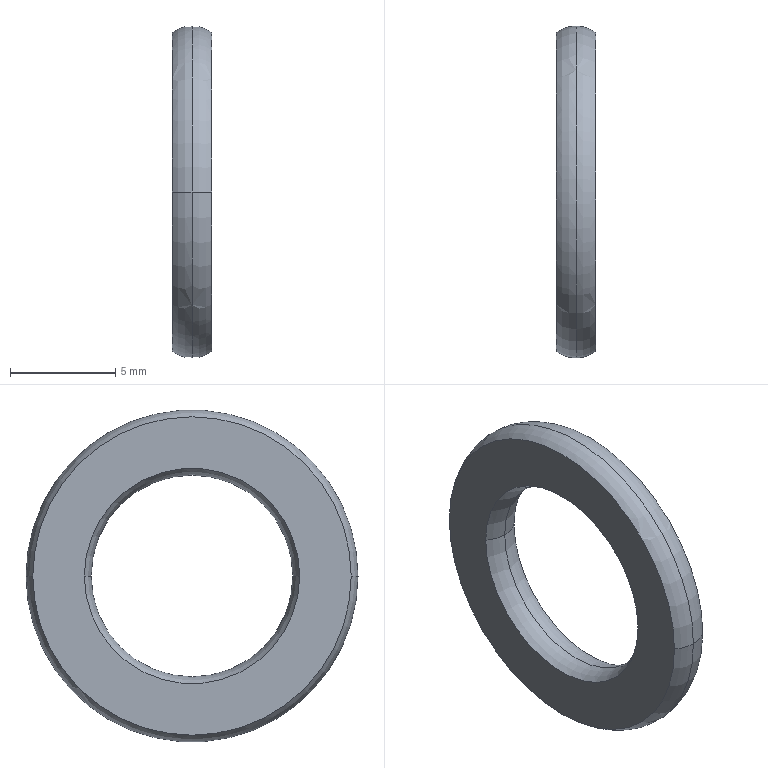Part | Creo | 1 solid | 10 faces | box 1.9 x 15.8 x 15.8 mm | volume 219.321 mm3 | torus 8 | plane 2
STEP:
#1=CARTESIAN_POINT('',(-128.,-90.537,-6.));
#2=VERTEX_POINT('',#1);
#3=CARTESIAN_POINT('',(-128.,-80.286,-6.));
#4=VERTEX_POINT('',#3);
#5=CARTESIAN_POINT('',(-128.,-85.411,-6.));
#6=DIRECTION('',(-1.,0.,0.));
#7=DIRECTION('',(0.,-1.,0.));
#8=AXIS2_PLACEMENT_3D('',#5,#6,#7);
#9=CIRCLE('',#8,5.125);
#10=EDGE_CURVE('',#2,#4,#9,.T.);
#11=ORIENTED_EDGE('',*,*,#10,.T.);
#12=CARTESIAN_POINT('',(-128.95,-80.611,-6.));
#13=VERTEX_POINT('',#12);
#14=CARTESIAN_POINT('',(-128.95,-79.061,-6.));
#15=DIRECTION('',(0.,0.,1.));
#16=DIRECTION('',(0.,-1.,0.));
#17=AXIS2_PLACEMENT_3D('',#14,#15,#16);
#18=CIRCLE('',#17,1.55);
#19=EDGE_CURVE('',#13,#4,#18,.T.);
#20=ORIENTED_EDGE('',*,*,#19,.F.);
#21=CARTESIAN_POINT('',(-128.95,-90.211,-6.));
#22=VERTEX_POINT('',#21);
#23=CARTESIAN_POINT('',(-128.95,-85.411,-6.));
#24=DIRECTION('',(-1.,0.,0.));
#25=DIRECTION('',(0.,-1.,0.));
#26=AXIS2_PLACEMENT_3D('',#23,#24,#25);
#27=CIRCLE('',#26,4.8);
#28=EDGE_CURVE('',#22,#13,#27,.T.);
#29=ORIENTED_EDGE('',*,*,#28,.F.);
#30=CARTESIAN_POINT('',(-128.95,-91.761,-6.));
#31=DIRECTION('',(0.,0.,-1.));
#32=DIRECTION('',(0.,1.,0.));
#33=AXIS2_PLACEMENT_3D('',#30,#31,#32);
#34=CIRCLE('',#33,1.55);
#35=EDGE_CURVE('',#22,#2,#34,.T.);
#36=ORIENTED_EDGE('',*,*,#35,.T.);
#37=EDGE_LOOP('',(#11,#20,#29,#36));
#38=FACE_OUTER_BOUND('',#37,.F.);
#39=CARTESIAN_POINT('',(-128.95,-85.411,-6.));
#40=DIRECTION('',(-1.,0.,0.));
#41=DIRECTION('',(0.,-1.,0.));
#42=AXIS2_PLACEMENT_3D('',#39,#40,#41);
#43=TOROIDAL_SURFACE('',#42,6.35,1.55);
#44=ADVANCED_FACE('',(#38),#43,.T.);
#45=CARTESIAN_POINT('',(-128.,-92.986,-6.));
#46=VERTEX_POINT('',#45);
#47=CARTESIAN_POINT('',(-128.,-77.837,-6.));
#48=VERTEX_POINT('',#47);
#49=CARTESIAN_POINT('',(-128.,-85.411,-6.));
#50=DIRECTION('',(1.,0.,0.));
#51=DIRECTION('',(0.,-1.,0.));
#52=AXIS2_PLACEMENT_3D('',#49,#50,#51);
#53=CIRCLE('',#52,7.575);
#54=EDGE_CURVE('',#46,#48,#53,.T.);
#55=ORIENTED_EDGE('',*,*,#54,.F.);
#56=CARTESIAN_POINT('',(-128.,-85.411,-6.));
#57=DIRECTION('',(1.,0.,0.));
#58=DIRECTION('',(0.,1.,0.));
#59=AXIS2_PLACEMENT_3D('',#56,#57,#58);
#60=CIRCLE('',#59,7.575);
#61=EDGE_CURVE('',#48,#46,#60,.T.);
#62=ORIENTED_EDGE('',*,*,#61,.F.);
#63=EDGE_LOOP('',(#55,#62));
#64=FACE_OUTER_BOUND('',#63,.F.);
#65=ORIENTED_EDGE('',*,*,#10,.F.);
#66=CARTESIAN_POINT('',(-128.,-85.411,-6.));
#67=DIRECTION('',(-1.,0.,0.));
#68=DIRECTION('',(0.,1.,0.));
#69=AXIS2_PLACEMENT_3D('',#66,#67,#68);
#70=CIRCLE('',#69,5.125);
#71=EDGE_CURVE('',#4,#2,#70,.T.);
#72=ORIENTED_EDGE('',*,*,#71,.F.);
#73=EDGE_LOOP('',(#65,#72));
#74=FACE_BOUND('',#73,.F.);
#75=CARTESIAN_POINT('',(-128.,-85.411,1.575));
#76=DIRECTION('',(1.,0.,0.));
#77=DIRECTION('',(0.,1.,0.));
#78=AXIS2_PLACEMENT_3D('',#75,#76,#77);
#79=PLANE('',#78);
#80=ADVANCED_FACE('',(#64,#74),#79,.T.);
#81=ORIENTED_EDGE('',*,*,#71,.T.);
#82=ORIENTED_EDGE('',*,*,#35,.F.);
#83=CARTESIAN_POINT('',(-128.95,-85.411,-6.));
#84=DIRECTION('',(-1.,0.,0.));
#85=DIRECTION('',(0.,1.,0.));
#86=AXIS2_PLACEMENT_3D('',#83,#84,#85);
#87=CIRCLE('',#86,4.8);
#88=EDGE_CURVE('',#13,#22,#87,.T.);
#89=ORIENTED_EDGE('',*,*,#88,.F.);
#90=ORIENTED_EDGE('',*,*,#19,.T.);
#91=EDGE_LOOP('',(#81,#82,#89,#90));
#92=FACE_OUTER_BOUND('',#91,.F.);
#93=CARTESIAN_POINT('',(-128.95,-85.411,-6.));
#94=DIRECTION('',(-1.,0.,0.));
#95=DIRECTION('',(0.,-1.,0.));
#96=AXIS2_PLACEMENT_3D('',#93,#94,#95);
#97=TOROIDAL_SURFACE('',#96,6.35,1.55);
#98=ADVANCED_FACE('',(#92),#97,.T.);
#99=CARTESIAN_POINT('',(-129.9,-90.537,-6.));
#100=VERTEX_POINT('',#99);
#101=CARTESIAN_POINT('',(-129.9,-80.286,-6.));
#102=VERTEX_POINT('',#101);
#103=CARTESIAN_POINT('',(-129.9,-85.411,-6.));
#104=DIRECTION('',(1.,0.,0.));
#105=DIRECTION('',(0.,-1.,0.));
#106=AXIS2_PLACEMENT_3D('',#103,#104,#105);
#107=CIRCLE('',#106,5.125);
#108=EDGE_CURVE('',#100,#102,#107,.T.);
#109=ORIENTED_EDGE('',*,*,#108,.T.);
#110=CARTESIAN_POINT('',(-128.95,-79.061,-6.));
#111=DIRECTION('',(0.,0.,1.));
#112=DIRECTION('',(-0.6129,-0.7902,0.));
#113=AXIS2_PLACEMENT_3D('',#110,#111,#112);
#114=CIRCLE('',#113,1.55);
#115=EDGE_CURVE('',#102,#13,#114,.T.);
#116=ORIENTED_EDGE('',*,*,#115,.T.);
#117=ORIENTED_EDGE('',*,*,#88,.T.);
#118=CARTESIAN_POINT('',(-128.95,-91.761,-6.));
#119=DIRECTION('',(0.,0.,-1.));
#120=DIRECTION('',(-0.6129,0.7902,0.));
#121=AXIS2_PLACEMENT_3D('',#118,#119,#120);
#122=CIRCLE('',#121,1.55);
#123=EDGE_CURVE('',#100,#22,#122,.T.);
#124=ORIENTED_EDGE('',*,*,#123,.F.);
#125=EDGE_LOOP('',(#109,#116,#117,#124));
#126=FACE_OUTER_BOUND('',#125,.F.);
#127=CARTESIAN_POINT('',(-128.95,-85.411,-6.));
#128=DIRECTION('',(-1.,0.,0.));
#129=DIRECTION('',(0.,-1.,0.));
#130=AXIS2_PLACEMENT_3D('',#127,#128,#129);
#131=TOROIDAL_SURFACE('',#130,6.35,1.55);
#132=ADVANCED_FACE('',(#126),#131,.T.);
#133=CARTESIAN_POINT('',(-129.9,-92.986,-6.));
#134=VERTEX_POINT('',#133);
#135=CARTESIAN_POINT('',(-129.9,-77.837,-6.));
#136=VERTEX_POINT('',#135);
#137=CARTESIAN_POINT('',(-129.9,-85.411,-6.));
#138=DIRECTION('',(-1.,0.,0.));
#139=DIRECTION('',(0.,-1.,0.));
#140=AXIS2_PLACEMENT_3D('',#137,#138,#139);
#141=CIRCLE('',#140,7.575);
#142=EDGE_CURVE('',#134,#136,#141,.T.);
#143=ORIENTED_EDGE('',*,*,#142,.F.);
#144=CARTESIAN_POINT('',(-129.9,-85.411,-6.));
#145=DIRECTION('',(-1.,0.,0.));
#146=DIRECTION('',(0.,1.,0.));
#147=AXIS2_PLACEMENT_3D('',#144,#145,#146);
#148=CIRCLE('',#147,7.575);
#149=EDGE_CURVE('',#136,#134,#148,.T.);
#150=ORIENTED_EDGE('',*,*,#149,.F.);
#151=EDGE_LOOP('',(#143,#150));
#152=FACE_OUTER_BOUND('',#151,.F.);
#153=ORIENTED_EDGE('',*,*,#108,.F.);
#154=CARTESIAN_POINT('',(-129.9,-85.411,-6.));
#155=DIRECTION('',(1.,0.,0.));
#156=DIRECTION('',(0.,1.,0.));
#157=AXIS2_PLACEMENT_3D('',#154,#155,#156);
#158=CIRCLE('',#157,5.125);
#159=EDGE_CURVE('',#102,#100,#158,.T.);
#160=ORIENTED_EDGE('',*,*,#159,.F.);
#161=EDGE_LOOP('',(#153,#160));
#162=FACE_BOUND('',#161,.F.);
#163=CARTESIAN_POINT('',(-129.9,-85.411,-0.8749));
#164=DIRECTION('',(-1.,0.,0.));
#165=DIRECTION('',(0.,-1.,0.));
#166=AXIS2_PLACEMENT_3D('',#163,#164,#165);
#167=PLANE('',#166);
#168=ADVANCED_FACE('',(#152,#162),#167,.T.);
#169=ORIENTED_EDGE('',*,*,#142,.T.);
#170=CARTESIAN_POINT('',(-128.95,-77.511,-6.));
#171=VERTEX_POINT('',#170);
#172=CARTESIAN_POINT('',(-128.95,-79.061,-6.));
#173=DIRECTION('',(0.,0.,1.));
#174=DIRECTION('',(0.,1.,0.));
#175=AXIS2_PLACEMENT_3D('',#172,#173,#174);
#176=CIRCLE('',#175,1.55);
#177=EDGE_CURVE('',#171,#136,#176,.T.);
#178=ORIENTED_EDGE('',*,*,#177,.F.);
#179=CARTESIAN_POINT('',(-128.95,-93.311,-6.));
#180=VERTEX_POINT('',#179);
#181=CARTESIAN_POINT('',(-128.95,-85.411,-6.));
#182=DIRECTION('',(-1.,0.,0.));
#183=DIRECTION('',(0.,-1.,0.));
#184=AXIS2_PLACEMENT_3D('',#181,#182,#183);
#185=CIRCLE('',#184,7.9);
#186=EDGE_CURVE('',#180,#171,#185,.T.);
#187=ORIENTED_EDGE('',*,*,#186,.F.);
#188=CARTESIAN_POINT('',(-128.95,-91.761,-6.));
#189=DIRECTION('',(0.,0.,-1.));
#190=DIRECTION('',(0.,-1.,0.));
#191=AXIS2_PLACEMENT_3D('',#188,#189,#190);
#192=CIRCLE('',#191,1.55);
#193=EDGE_CURVE('',#180,#134,#192,.T.);
#194=ORIENTED_EDGE('',*,*,#193,.T.);
#195=EDGE_LOOP('',(#169,#178,#187,#194));
#196=FACE_OUTER_BOUND('',#195,.F.);
#197=CARTESIAN_POINT('',(-128.95,-85.411,-6.));
#198=DIRECTION('',(-1.,0.,0.));
#199=DIRECTION('',(0.,-1.,0.));
#200=AXIS2_PLACEMENT_3D('',#197,#198,#199);
#201=TOROIDAL_SURFACE('',#200,6.35,1.55);
#202=ADVANCED_FACE('',(#196),#201,.T.);
#203=ORIENTED_EDGE('',*,*,#149,.T.);
#204=ORIENTED_EDGE('',*,*,#193,.F.);
#205=CARTESIAN_POINT('',(-128.95,-85.411,-6.));
#206=DIRECTION('',(-1.,0.,0.));
#207=DIRECTION('',(0.,1.,0.));
#208=AXIS2_PLACEMENT_3D('',#205,#206,#207);
#209=CIRCLE('',#208,7.9);
#210=EDGE_CURVE('',#171,#180,#209,.T.);
#211=ORIENTED_EDGE('',*,*,#210,.F.);
#212=ORIENTED_EDGE('',*,*,#177,.T.);
#213=EDGE_LOOP('',(#203,#204,#211,#212));
#214=FACE_OUTER_BOUND('',#213,.F.);
#215=CARTESIAN_POINT('',(-128.95,-85.411,-6.));
#216=DIRECTION('',(-1.,0.,0.));
#217=DIRECTION('',(0.,-1.,0.));
#218=AXIS2_PLACEMENT_3D('',#215,#216,#217);
#219=TOROIDAL_SURFACE('',#218,6.35,1.55);
#220=ADVANCED_FACE('',(#214),#219,.T.);
#221=ORIENTED_EDGE('',*,*,#54,.T.);
#222=CARTESIAN_POINT('',(-128.95,-79.061,-6.));
#223=DIRECTION('',(0.,0.,1.));
#224=DIRECTION('',(0.6129,0.7902,0.));
#225=AXIS2_PLACEMENT_3D('',#222,#223,#224);
#226=CIRCLE('',#225,1.55);
#227=EDGE_CURVE('',#48,#171,#226,.T.);
#228=ORIENTED_EDGE('',*,*,#227,.T.);
#229=ORIENTED_EDGE('',*,*,#210,.T.);
#230=CARTESIAN_POINT('',(-128.95,-91.761,-6.));
#231=DIRECTION('',(0.,0.,-1.));
#232=DIRECTION('',(0.6129,-0.7902,0.));
#233=AXIS2_PLACEMENT_3D('',#230,#231,#232);
#234=CIRCLE('',#233,1.55);
#235=EDGE_CURVE('',#46,#180,#234,.T.);
#236=ORIENTED_EDGE('',*,*,#235,.F.);
#237=EDGE_LOOP('',(#221,#228,#229,#236));
#238=FACE_OUTER_BOUND('',#237,.F.);
#239=CARTESIAN_POINT('',(-128.95,-85.411,-6.));
#240=DIRECTION('',(-1.,0.,0.));
#241=DIRECTION('',(0.,-1.,0.));
#242=AXIS2_PLACEMENT_3D('',#239,#240,#241);
#243=TOROIDAL_SURFACE('',#242,6.35,1.55);
#244=ADVANCED_FACE('',(#238),#243,.T.);
#245=ORIENTED_EDGE('',*,*,#61,.T.);
#246=ORIENTED_EDGE('',*,*,#235,.T.);
#247=ORIENTED_EDGE('',*,*,#186,.T.);
#248=ORIENTED_EDGE('',*,*,#227,.F.);
#249=EDGE_LOOP('',(#245,#246,#247,#248));
#250=FACE_OUTER_BOUND('',#249,.F.);
#251=CARTESIAN_POINT('',(-128.95,-85.411,-6.));
#252=DIRECTION('',(-1.,0.,0.));
#253=DIRECTION('',(0.,-1.,0.));
#254=AXIS2_PLACEMENT_3D('',#251,#252,#253);
#255=TOROIDAL_SURFACE('',#254,6.35,1.55);
#256=ADVANCED_FACE('',(#250),#255,.T.);
#257=ORIENTED_EDGE('',*,*,#159,.T.);
#258=ORIENTED_EDGE('',*,*,#123,.T.);
#259=ORIENTED_EDGE('',*,*,#28,.T.);
#260=ORIENTED_EDGE('',*,*,#115,.F.);
#261=EDGE_LOOP('',(#257,#258,#259,#260));
#262=FACE_OUTER_BOUND('',#261,.F.);
#263=CARTESIAN_POINT('',(-128.95,-85.411,-6.));
#264=DIRECTION('',(-1.,0.,0.));
#265=DIRECTION('',(0.,-1.,0.));
#266=AXIS2_PLACEMENT_3D('',#263,#264,#265);
#267=TOROIDAL_SURFACE('',#266,6.35,1.55);
#268=ADVANCED_FACE('',(#262),#267,.T.);
#269=CLOSED_SHELL('',(#44,#80,#98,#132,#168,#202,#220,#244,#256,#268));
#270=MANIFOLD_SOLID_BREP('',#269);
#271=(LENGTH_UNIT()NAMED_UNIT(*)SI_UNIT(.MILLI.,.METRE.));
#272=UNCERTAINTY_MEASURE_WITH_UNIT(LENGTH_MEASURE(0.002242),#271,'','');
#273=(NAMED_UNIT(*)PLANE_ANGLE_UNIT()SI_UNIT($,.RADIAN.));
#274=PLANE_ANGLE_MEASURE_WITH_UNIT(PLANE_ANGLE_MEASURE(0.01745),#273);
#275=(CONVERSION_BASED_UNIT('DEGREE',#274)NAMED_UNIT(*)PLANE_ANGLE_UNIT());
#276=(NAMED_UNIT(*)SI_UNIT($,.STERADIAN.)SOLID_ANGLE_UNIT());
#277=(GEOMETRIC_REPRESENTATION_CONTEXT(3)GLOBAL_UNCERTAINTY_ASSIGNED_CONTEXT((#272))GLOBAL_UNIT_ASSIGNED_CONTEXT((#271,#275,#276))REPRESENTATION_CONTEXT('',''));
#278=ADVANCED_BREP_SHAPE_REPRESENTATION('',(#270),#277);